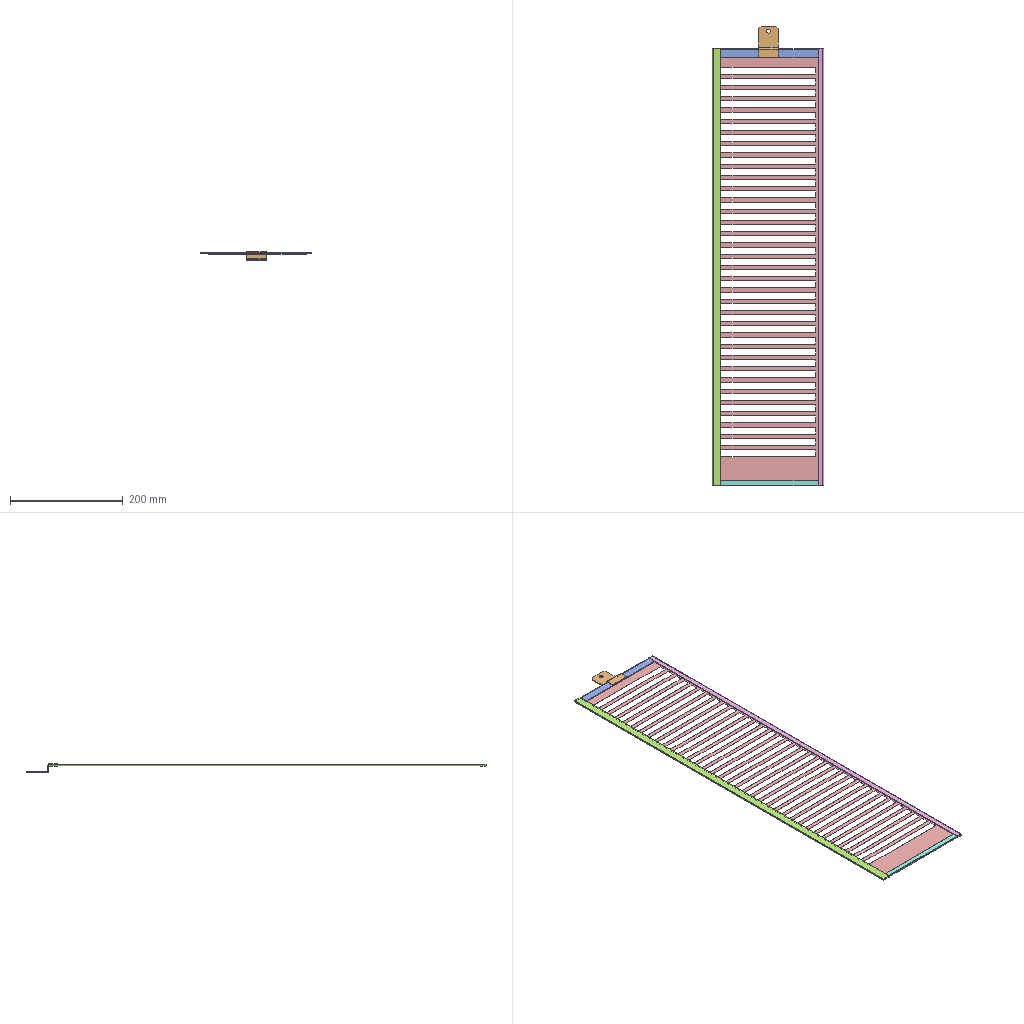Assembly | SolidWorks | 6 different items | 6 placed | box 198 x 818 x 16 mm
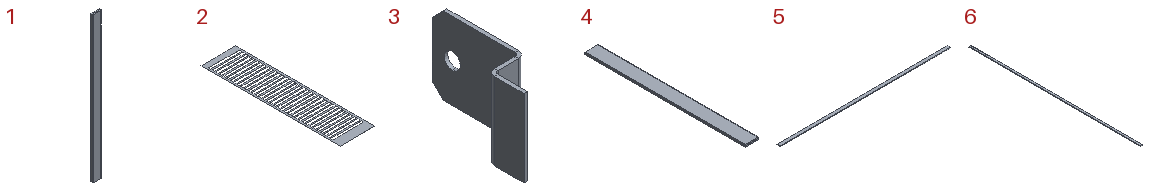Parts list (item | quantity | size | volume | features):
1 | x1 | 10 x 2.7 x 173.1 mm | 4083 mm3 | features FlatPattern 1, Hem 1, ICE 1, SMBaseFlange 1, SheetMetal 1
2 | x1 | 194.4 x 773 x 0.26 mm | 19811 mm3 | features FlatPattern 1, ICE 1, SMBaseFlange 1, SheetMetal 1
3 | x1 | 15.7 x 55.6 x 35 mm | 3683 mm3 | features Chamfer 2, FlatPattern 1, ICE 1, SMBaseFlange 1, SheetMetal 1
4 | x1 | 15 x 173.1 x 2.7 mm | 6160 mm3 | features FlatPattern 1, Hem 1, SMBaseFlange 1, SheetMetal 1
5 | x1 | 777 x 15 x 2.7 mm | 27651 mm3 | features FlatPattern 1, Hem 1, SMBaseFlange 1, SheetMetal 1
6 | x1 | 10 x 777 x 2.7 mm | 18327 mm3 | features FlatPattern 1, Hem 1, SMBaseFlange 1, SheetMetal 1
Mates (type | each side: item.copy, entity, surface, feature):
Parallel | 2.1 face plane Base-Flange1 | 4.1 face plane Base-Flange1 | 2 times
DistanceDim | 4.1 face plane Base-Flange1 | 2.1 face plane Base-Flange1
DistanceDim | 4.1 face plane Hem1 | 2.1 face plane Base-Flange1
Parallel | 2.1 face plane Base-Flange1 | 5.1 face plane Hem1 | 2 times
Coincident | 2.1 face plane Base-Flange1 | 5.1 face plane Hem1
DistanceDim | 2.1 edge | 4.1 edge
DistanceDim | 5.1 edge | 4.1 edge
Parallel | 2.1 face plane Base-Flange1 | 6.1 face plane Base-Flange1 | 2 times
Coincident | 2.1 face plane Base-Flange1 | 6.1 face plane Base-Flange1
DistanceDim | 6.1 edge | 4.1 edge
Coincident | 4.1 face plane Hem1 | 6.1 face plane Base-Flange1
Coincident | 4.1 face plane Hem1 | 5.1 face plane Hem1
Parallel | 2.1 face plane Base-Flange1 | 1.1 face plane Hem1
Parallel | 2.1 face plane Base-Flange1 | 1.1 face plane Base-Flange1
DistanceDim | 1.1 face plane Base-Flange1 | 2.1 face plane Base-Flange1
DistanceDim | 5.1 edge | 1.1 edge
Coincident | 5.1 face plane Base-Flange1 | 1.1 face plane Cut-Extrude2
Coincident | 4.1 face plane Base-Flange1 | 3.1 face plane Base-Flange1
DistanceDim | 3.1 face plane Base-Flange1 | 4.1 face plane Base-Flange1
DistanceDim | 6.1 edge | 3.1 edge